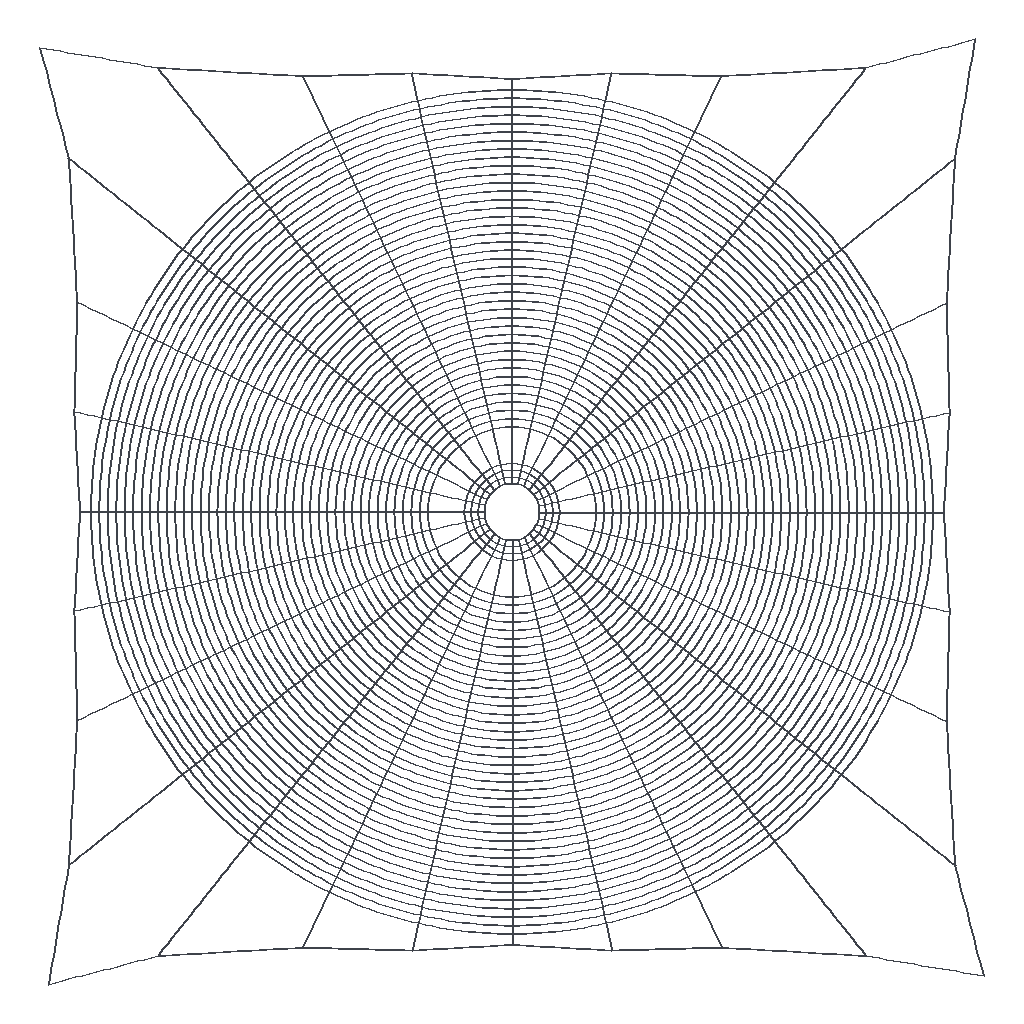Simulation study | abaqus
Set-up summary:
category,name,step,type,value,unit,region
solver,abaqus
solver,version,,,Abaqus/Explicit 2020
units,not stated in the deck,,not stated
analysis,deck,,transient,transient
load_step,Step-1,Step-1,transient,nlgeom=True
contact,interactions,,,general=0 pairs=0 ties=0
load_step,requested,,,1
mesh,nodes,,,10068
mesh,elements,,,11328
element_type,T3D2,,truss,11328
load,load commands in deck,,count,1
bc,support commands in deck,,count,1
material,MATERIAL-1,,in results
check,setup vs results,,match,"per instance, exact: element labels, types and connectivity; labels of the nodes the elements use; coordinates of those nodes at SINGLE_PRECISION in 1 of 1 instance(s)"
Abaqus input file, long lists of numbers shortened:
*Heading
** Job name: Job-1 Model name: Model-1
** Generated by: Abaqus/CAE 2020
*Preprint, echo=NO, model=NO, history=NO, contact=NO
**
** PARTS
**
*Part, name=busi
*Node
      1,  -124.308,   258.128,           0.
      2,  -108.47,   225.243,           0.
** (10066 more lines like these left out)
*Element, type=T3D2
1,    1, 1338
2, 1338, 1339
** (11326 more lines like these left out)
*Nset, nset=Set-1, generate
     1,  10068,      1
*Elset, elset=Set-1, generate
     1,  11328,      1
** Section: Section-1
*Solid Section, elset=Set-1, material=Material-1
1.,
*End Part
**
**
** ASSEMBLY
**
*Assembly, name=Assembly
**
*Instance, name=busi-1, part=busi
*End Instance
**
*Nset, nset=Set-1, instance=busi-1
   93,  278,  324,  372,  464,  465,  842,  843,  844,  849,  850,  851, 2890, 2891, 2892, 2893
 2894, 2895, 2896, 2897, 2898, 2899, 2900, 2901, 2902, 2903, 2904, 2905, 3575, 3576, 3577, 3578
** (7 more lines like these left out)
*Elset, elset=Set-1, instance=busi-1
 2054, 2055, 2056, 2057, 2058, 2059, 2060, 2061, 2062, 2063, 2064, 2065, 2066, 2067, 2068, 2069
 2070, 2924, 2925, 2926, 2927, 2928, 2929, 2930, 2931, 2932, 2933, 2934, 2935, 2936, 2937, 2938
** (7 more lines like these left out)
*Nset, nset=Set-2, instance=busi-1
 496,
*Nset, nset=Set-3, instance=busi-1, generate
 495,  497,    1
*End Assembly
*Amplitude, name=Amp-1
             0.,              0.,              1.,              1.
**
** MATERIALS
**
*Material, name=Material-1
*Density
 5e-10,
*Elastic
600., 0.4
*Plastic
 10.,  0.
200., 0.4
** ----------------------------------------------------------------
**
** STEP: Step-1
**
*Step, name=Step-1, nlgeom=YES
*Dynamic, Explicit
, 0.01
*Bulk Viscosity
0.06, 1.2
**
** BOUNDARY CONDITIONS
**
** Name: BC-1 Type: 对称/反对称/完全固定
*Boundary
Set-1, ENCASTRE
**
** LOADS
**
** Name: Load-1   Type: Concentrated force
*Cload
Set-3, 3, -10.
**
** OUTPUT REQUESTS
**
*Restart, write, number interval=1, time marks=NO
**
** FIELD OUTPUT: F-Output-1
**
*Output, field
*Node Output
CF, RF, U, V
*Element Output, directions=YES
E, LE, MISES, PE, PEEQ, PEMAG, S
*Contact Output
CDISP, CSTRESS
**
** HISTORY OUTPUT: H-Output-1
**
*Output, history, variable=PRESELECT, frequency=1
*End Step
Results summary:
result,step,Step-1,completed,increments=19044 time=0.01/0.01
result,analysis,,,transient
result,last_loadstep,,,1
result,analysis steps,,count,1
result,primary field,,,U
result,reaction total,,FX,4.853,model units
result,reaction total,,FY,3.627,model units
result,reaction total,,FZ,47.45,model units